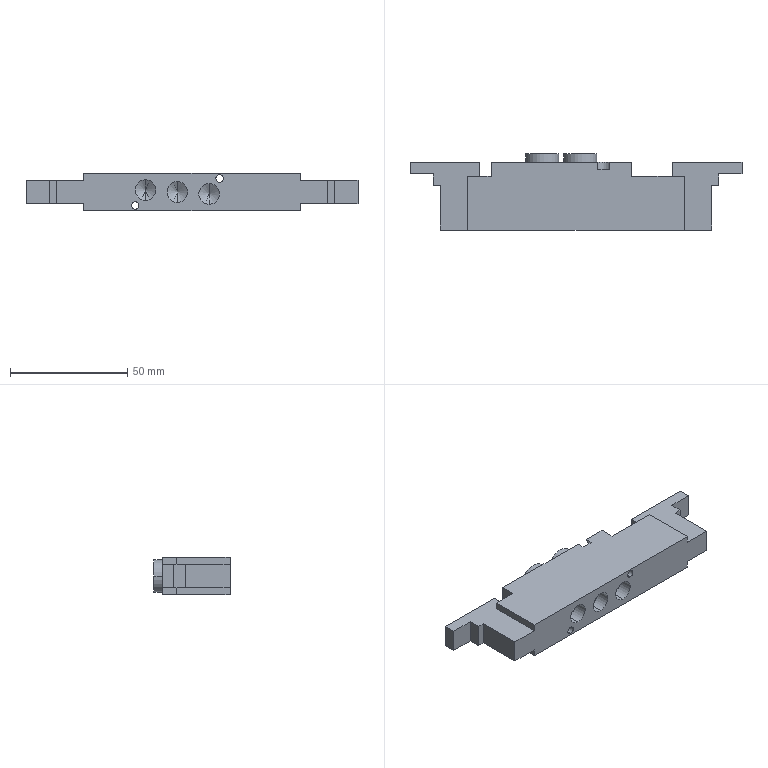Part | STEP file | Solenoid valve 7V130C06B-NS | 1 solid | 71 faces | box 141.7 x 32.5 x 16 mm | volume 47379 mm3 | plane 36 | cylinder 25 | cone 10 | commonest cylinder face diameters 8.8 x6 2.5 x4 3.2 x4 10 x4 14 x4 6.5 x3